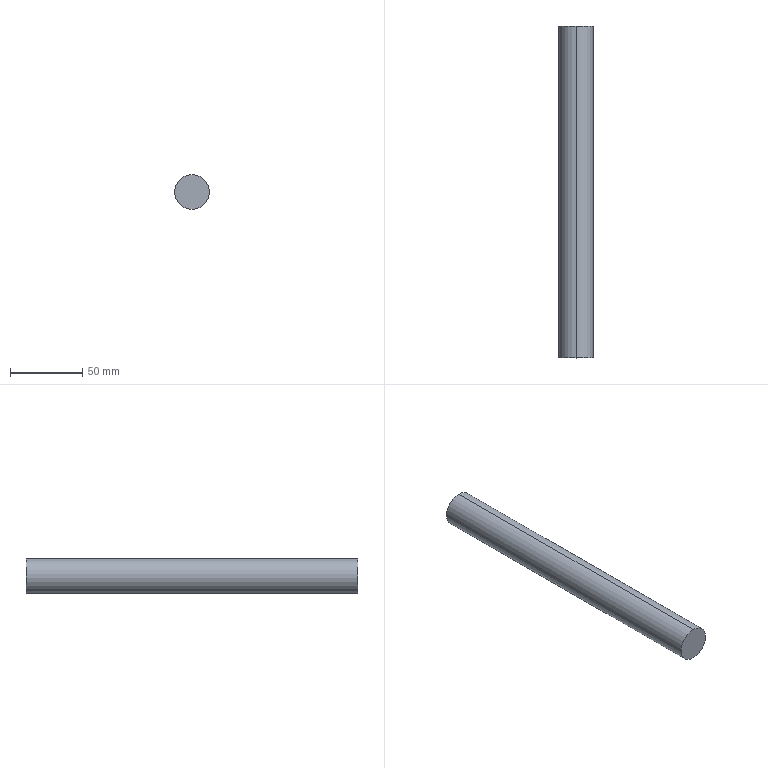Part | SolidWorks | features BaseBody 1 | 1 solid | 4 faces | box 24 x 230 x 24 mm | volume 104050 mm3 | cylinder 2 | plane 2 | commonest cylinder face diameters 24 x2
STEP:
#1=CARTESIAN_POINT('',(0.,230.,-12.));
#2=VERTEX_POINT('',#1);
#3=CARTESIAN_POINT('',(0.,230.,12.));
#4=VERTEX_POINT('',#3);
#5=CARTESIAN_POINT('',(0.,230.,0.));
#6=DIRECTION('',(0.,-1.,0.));
#7=DIRECTION('',(0.,0.,-1.));
#8=AXIS2_PLACEMENT_3D('',#5,#6,#7);
#9=CIRCLE('',#8,12.);
#10=EDGE_CURVE('',#2,#4,#9,.T.);
#11=ORIENTED_EDGE('',*,*,#10,.T.);
#12=CARTESIAN_POINT('',(0.,0.,12.));
#13=VERTEX_POINT('',#12);
#14=CARTESIAN_POINT('',(0.,230.,12.));
#15=DIRECTION('',(0.,-1.,0.));
#16=VECTOR('',#15,1000.);
#17=LINE('',#14,#16);
#18=EDGE_CURVE('',#4,#13,#17,.T.);
#19=ORIENTED_EDGE('',*,*,#18,.T.);
#20=CARTESIAN_POINT('',(0.,0.,-12.));
#21=VERTEX_POINT('',#20);
#22=CARTESIAN_POINT('',(0.,0.,0.));
#23=DIRECTION('',(0.,1.,0.));
#24=DIRECTION('',(0.,0.,-1.));
#25=AXIS2_PLACEMENT_3D('',#22,#23,#24);
#26=CIRCLE('',#25,12.);
#27=EDGE_CURVE('',#13,#21,#26,.T.);
#28=ORIENTED_EDGE('',*,*,#27,.T.);
#29=CARTESIAN_POINT('',(0.,230.,-12.));
#30=DIRECTION('',(0.,-1.,0.));
#31=VECTOR('',#30,1000.);
#32=LINE('',#29,#31);
#33=EDGE_CURVE('',#2,#21,#32,.T.);
#34=ORIENTED_EDGE('',*,*,#33,.F.);
#35=EDGE_LOOP('',(#11,#19,#28,#34));
#36=FACE_OUTER_BOUND('',#35,.T.);
#37=CARTESIAN_POINT('',(0.,230.,0.));
#38=DIRECTION('',(0.,-1.,0.));
#39=DIRECTION('',(0.,0.,-1.));
#40=AXIS2_PLACEMENT_3D('',#37,#38,#39);
#41=CYLINDRICAL_SURFACE('',#40,12.);
#42=ADVANCED_FACE('',(#36),#41,.T.);
#43=ORIENTED_EDGE('',*,*,#18,.F.);
#44=CARTESIAN_POINT('',(0.,230.,0.));
#45=DIRECTION('',(0.,-1.,0.));
#46=DIRECTION('',(0.,0.,-1.));
#47=AXIS2_PLACEMENT_3D('',#44,#45,#46);
#48=CIRCLE('',#47,12.);
#49=EDGE_CURVE('',#4,#2,#48,.T.);
#50=ORIENTED_EDGE('',*,*,#49,.T.);
#51=ORIENTED_EDGE('',*,*,#33,.T.);
#52=CARTESIAN_POINT('',(0.,0.,0.));
#53=DIRECTION('',(0.,1.,0.));
#54=DIRECTION('',(0.,0.,-1.));
#55=AXIS2_PLACEMENT_3D('',#52,#53,#54);
#56=CIRCLE('',#55,12.);
#57=EDGE_CURVE('',#21,#13,#56,.T.);
#58=ORIENTED_EDGE('',*,*,#57,.T.);
#59=EDGE_LOOP('',(#43,#50,#51,#58));
#60=FACE_OUTER_BOUND('',#59,.T.);
#61=CARTESIAN_POINT('',(0.,230.,0.));
#62=DIRECTION('',(0.,-1.,0.));
#63=DIRECTION('',(0.,0.,-1.));
#64=AXIS2_PLACEMENT_3D('',#61,#62,#63);
#65=CYLINDRICAL_SURFACE('',#64,12.);
#66=ADVANCED_FACE('',(#60),#65,.T.);
#67=ORIENTED_EDGE('',*,*,#57,.F.);
#68=ORIENTED_EDGE('',*,*,#27,.F.);
#69=EDGE_LOOP('',(#67,#68));
#70=FACE_OUTER_BOUND('',#69,.T.);
#71=CARTESIAN_POINT('',(0.,0.,0.));
#72=DIRECTION('',(0.,1.,0.));
#73=DIRECTION('',(0.,0.,1.));
#74=AXIS2_PLACEMENT_3D('',#71,#72,#73);
#75=PLANE('',#74);
#76=ADVANCED_FACE('',(#70),#75,.F.);
#77=ORIENTED_EDGE('',*,*,#10,.F.);
#78=ORIENTED_EDGE('',*,*,#49,.F.);
#79=EDGE_LOOP('',(#77,#78));
#80=FACE_OUTER_BOUND('',#79,.T.);
#81=CARTESIAN_POINT('',(0.,230.,0.));
#82=DIRECTION('',(0.,1.,0.));
#83=DIRECTION('',(0.,0.,1.));
#84=AXIS2_PLACEMENT_3D('',#81,#82,#83);
#85=PLANE('',#84);
#86=ADVANCED_FACE('',(#80),#85,.T.);
#87=CLOSED_SHELL('',(#42,#66,#76,#86));
#88=MANIFOLD_SOLID_BREP('',#87);
#89=CARTESIAN_POINT('',(0.,0.,0.));
#90=DIRECTION('',(0.,0.,1.));
#91=DIRECTION('',(1.,0.,0.));
#92=AXIS2_PLACEMENT_3D('',#89,#90,#91);
#93=(LENGTH_UNIT()NAMED_UNIT(*)SI_UNIT(.MILLI.,.METRE.));
#94=UNCERTAINTY_MEASURE_WITH_UNIT(LENGTH_MEASURE(0.00001),#93,'','');
#95=(NAMED_UNIT(*)PLANE_ANGLE_UNIT()SI_UNIT($,.RADIAN.));
#96=(NAMED_UNIT(*)SI_UNIT($,.STERADIAN.)SOLID_ANGLE_UNIT());
#97=(GEOMETRIC_REPRESENTATION_CONTEXT(3)GLOBAL_UNCERTAINTY_ASSIGNED_CONTEXT((#94))GLOBAL_UNIT_ASSIGNED_CONTEXT((#93,#95,#96))REPRESENTATION_CONTEXT('',''));
#98=ADVANCED_BREP_SHAPE_REPRESENTATION('',(#88,#92),#97);